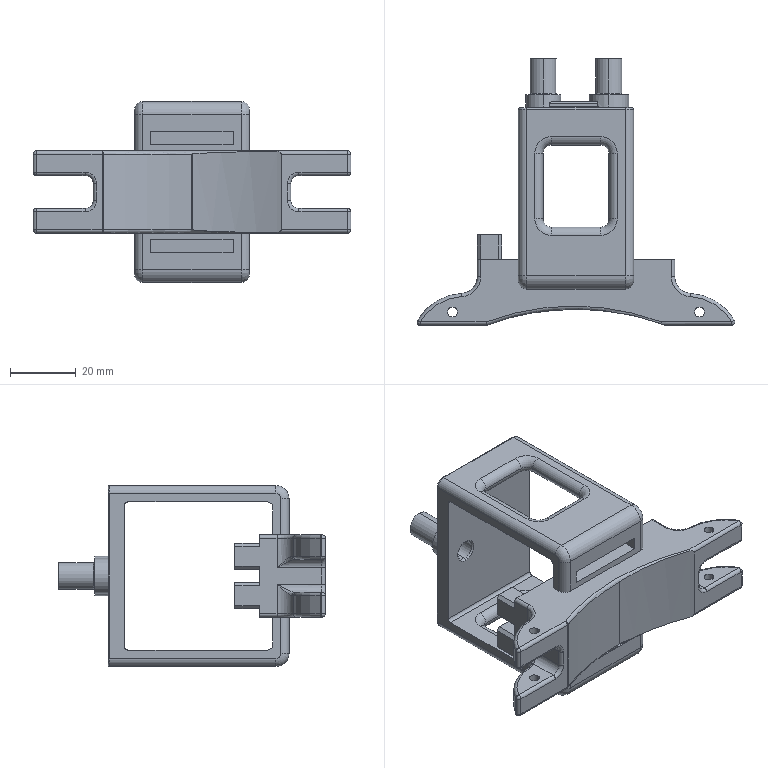Part | SolidWorks | features ICE 16, Fillet 10, MirrorPattern 3, Chamfer 2, 3DProfileFeature 1, Extrusion 1, HoleWzd 1, Scale 1 | 1 solid | 271 faces | box 96.57 x 80.995 x 55 mm | volume 46597 mm3 | cylinder 110 | plane 77 | torus 46 | cone 20 | sphere 14 | spline 4 | commonest cylinder face diameters 2 x28 5 x28 1 x12 3 x10 1.65 x8 8 x6